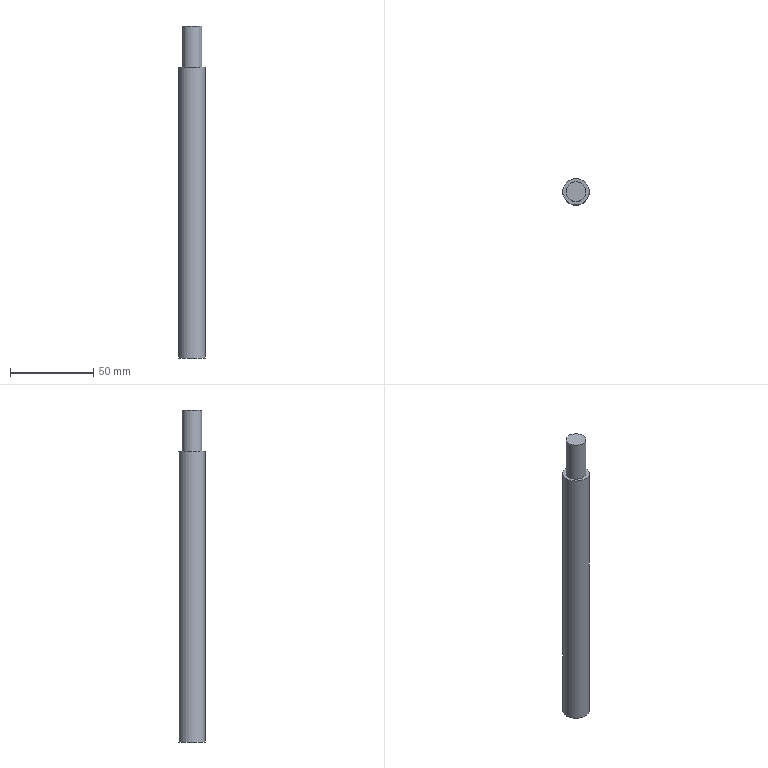Part | NX | features solid 2 | 1 solid | 5 faces | box 16 x 16 x 200 mm | volume 38013 mm3 | plane 3 | cylinder 2 | commonest cylinder face diameters 12 x1 16 x1
STEP:
#1=CARTESIAN_POINT('',(678.,10.,-75.));
#2=VERTEX_POINT('',#1);
#3=CARTESIAN_POINT('',(670.,10.,-75.));
#4=DIRECTION('',(0.,0.,1.));
#5=DIRECTION('',(1.,0.,0.));
#6=AXIS2_PLACEMENT_3D('',#3,#4,#5);
#7=CIRCLE('',#6,8.);
#8=EDGE_CURVE('',#2,#2,#7,.T.);
#9=ORIENTED_EDGE('',*,*,#8,.T.);
#10=EDGE_LOOP('',(#9));
#11=FACE_BOUND('',#10,.T.);
#12=CARTESIAN_POINT('',(676.,10.,-75.));
#13=VERTEX_POINT('',#12);
#14=CARTESIAN_POINT('',(670.,10.,-75.));
#15=DIRECTION('',(0.,0.,1.));
#16=DIRECTION('',(1.,0.,0.));
#17=AXIS2_PLACEMENT_3D('',#14,#15,#16);
#18=CIRCLE('',#17,6.);
#19=EDGE_CURVE('',#13,#13,#18,.T.);
#20=ORIENTED_EDGE('',*,*,#19,.F.);
#21=EDGE_LOOP('',(#20));
#22=FACE_BOUND('',#21,.T.);
#23=CARTESIAN_POINT('',(585.,225.,-75.));
#24=DIRECTION('',(0.,0.,1.));
#25=DIRECTION('',(1.,0.,0.));
#26=AXIS2_PLACEMENT_3D('',#23,#24,#25);
#27=PLANE('',#26);
#28=ADVANCED_FACE('',(#11,#22),#27,.T.);
#29=CARTESIAN_POINT('',(678.,10.,-250.));
#30=VERTEX_POINT('',#29);
#31=CARTESIAN_POINT('',(670.,10.,-250.));
#32=DIRECTION('',(0.,0.,1.));
#33=DIRECTION('',(1.,0.,0.));
#34=AXIS2_PLACEMENT_3D('',#31,#32,#33);
#35=CIRCLE('',#34,8.);
#36=EDGE_CURVE('',#30,#30,#35,.T.);
#37=ORIENTED_EDGE('',*,*,#36,.T.);
#38=EDGE_LOOP('',(#37));
#39=FACE_BOUND('',#38,.T.);
#40=ORIENTED_EDGE('',*,*,#8,.F.);
#41=EDGE_LOOP('',(#40));
#42=FACE_BOUND('',#41,.T.);
#43=CARTESIAN_POINT('',(670.,10.,-10.));
#44=DIRECTION('',(0.,0.,-1.));
#45=DIRECTION('',(-1.,0.,0.));
#46=AXIS2_PLACEMENT_3D('',#43,#44,#45);
#47=CYLINDRICAL_SURFACE('',#46,8.);
#48=ADVANCED_FACE('',(#39,#42),#47,.T.);
#49=ORIENTED_EDGE('',*,*,#36,.F.);
#50=EDGE_LOOP('',(#49));
#51=FACE_BOUND('',#50,.T.);
#52=CARTESIAN_POINT('',(670.,10.,-250.));
#53=DIRECTION('',(0.,0.,1.));
#54=DIRECTION('',(1.,0.,0.));
#55=AXIS2_PLACEMENT_3D('',#52,#53,#54);
#56=PLANE('',#55);
#57=ADVANCED_FACE('',(#51),#56,.F.);
#58=CARTESIAN_POINT('',(664.,10.,-50.));
#59=VERTEX_POINT('',#58);
#60=CARTESIAN_POINT('',(670.,10.,-50.));
#61=DIRECTION('',(0.,0.,-1.));
#62=DIRECTION('',(-1.,0.,0.));
#63=AXIS2_PLACEMENT_3D('',#60,#61,#62);
#64=CIRCLE('',#63,6.);
#65=EDGE_CURVE('',#59,#59,#64,.F.);
#66=ORIENTED_EDGE('',*,*,#65,.T.);
#67=EDGE_LOOP('',(#66));
#68=FACE_BOUND('',#67,.T.);
#69=CARTESIAN_POINT('',(585.,225.,-50.));
#70=DIRECTION('',(0.,0.,-1.));
#71=DIRECTION('',(0.,1.,0.));
#72=AXIS2_PLACEMENT_3D('',#69,#70,#71);
#73=PLANE('',#72);
#74=ADVANCED_FACE('',(#68),#73,.F.);
#75=ORIENTED_EDGE('',*,*,#19,.T.);
#76=EDGE_LOOP('',(#75));
#77=FACE_BOUND('',#76,.T.);
#78=ORIENTED_EDGE('',*,*,#65,.F.);
#79=EDGE_LOOP('',(#78));
#80=FACE_BOUND('',#79,.T.);
#81=CARTESIAN_POINT('',(670.,10.,-10.));
#82=DIRECTION('',(0.,0.,-1.));
#83=DIRECTION('',(-1.,0.,0.));
#84=AXIS2_PLACEMENT_3D('',#81,#82,#83);
#85=CYLINDRICAL_SURFACE('',#84,6.);
#86=ADVANCED_FACE('',(#77,#80),#85,.T.);
#87=CLOSED_SHELL('',(#28,#48,#57,#74,#86));
#88=MANIFOLD_SOLID_BREP('',#87);
#89=(LENGTH_UNIT()NAMED_UNIT(*)SI_UNIT(.MILLI.,.METRE.));
#90=UNCERTAINTY_MEASURE_WITH_UNIT(LENGTH_MEASURE(0.00001),#89,'','');
#91=(NAMED_UNIT(*)PLANE_ANGLE_UNIT()SI_UNIT($,.RADIAN.));
#92=(NAMED_UNIT(*)SI_UNIT($,.STERADIAN.)SOLID_ANGLE_UNIT());
#93=(GEOMETRIC_REPRESENTATION_CONTEXT(3)GLOBAL_UNCERTAINTY_ASSIGNED_CONTEXT((#90))GLOBAL_UNIT_ASSIGNED_CONTEXT((#89,#91,#92))REPRESENTATION_CONTEXT('',''));
#94=ADVANCED_BREP_SHAPE_REPRESENTATION('',(#88),#93);